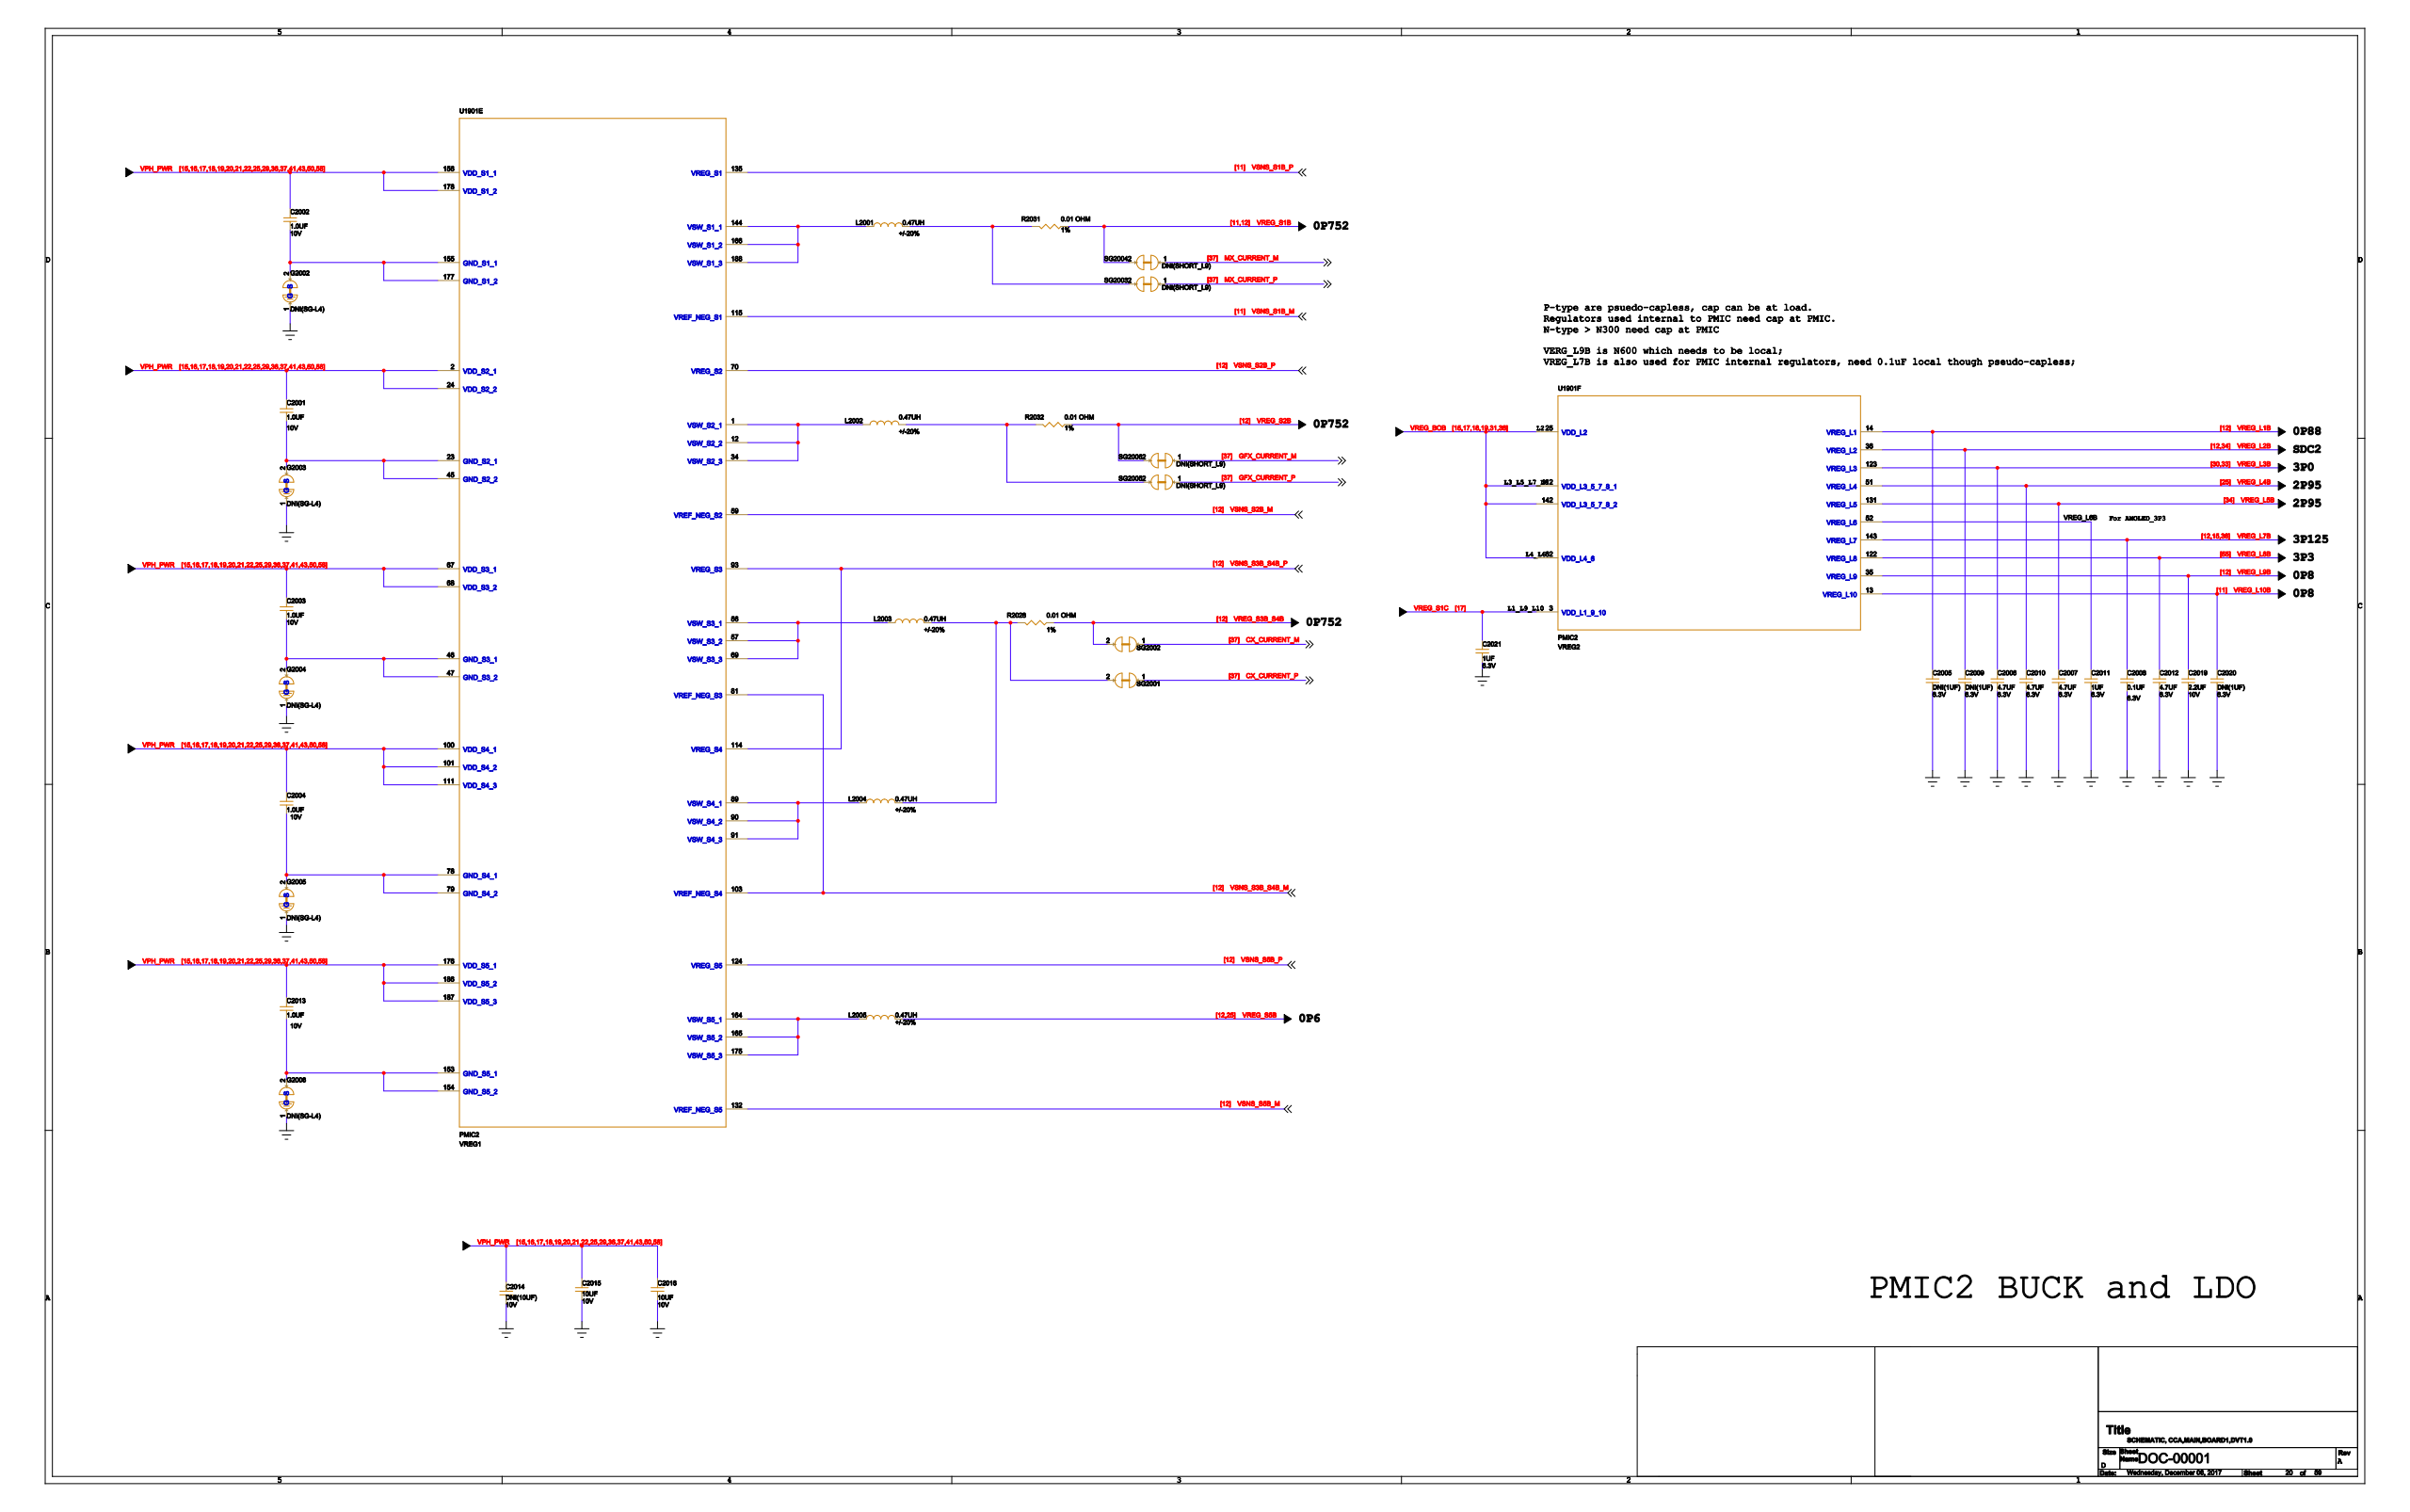Circuit board | KiCad | 1657 parts | 1365 nets | one sheet of the schematic
Parts on this sheet (reference | value | footprint):
C2001
C2002
C2003
C2004
C2005
C2006
C2007
C2008
C2009
C2010
C2011
C2012
C2013
C2014
C2015
C2016
C2019
C2020
C2021
G2002
G2003
G2004
G2005
G2006
L2001
L2002
L2003
L2004
L2005
R2028
R2031
R2032
SG2001
SG2002
SG2003
SG2004
SG2005
SG2006
U1901
Nets of these parts (net: part-pin ...):
GND: C2005-1 C2006-1 C2007-1 C2008-1 C2009-1 C2010-1 C2011-1 C2012-1 C2014-1 C2015-1 C2016-1 C2019-1 C2020-1 C2021-2 G2002-1 G2003-1 G2004-1 G2005-1 G2006-1
VPH_PWR: C2001-2 C2002-2 C2003-2 C2004-2 C2013-2 C2014-2 C2015-2 C2016-2 U1901-2 U1901-17 U1901-21 U1901-24 U1901-67 U1901-68 U1901-100 U1901-101 U1901-111 U1901-156 U1901-176 U1901-178 U1901-186 U1901-187
VREG_L2B: C2009-2 U1901-36
VSNS_S3B_S4B_M: U1901-81 U1901-103
VREG_BOB: U1901-20 U1901-25 U1901-41 U1901-62 U1901-112 U1901-142
VREG_L8B: C2012-2 U1901-122
VREG_S2B: R2032-2 SG2006-2
VSNS_S2B_P: U1901-70
VREG_L7B: C2008-2 U1901-143
N41047485: C2001-1 G2003-2 U1901-23 U1901-45
VREG_L5B: C2007-2 U1901-131
CX_CURRENT_M: SG2002-1
VREG_S3B_S4B: R2028-2 SG2002-2
VSNS_S1B_M: U1901-115
CX_CURRENT_P: SG2001-1
N22195111: L2003-2 L2004-2 R2028-1 SG2001-2
VREG_L4B: C2010-2 U1901-51
VREG_L10B: C2020-2 U1901-13
N41047633: C2003-1 G2004-2 U1901-46 U1901-47
VSNS_S5B_M: U1901-132
N41047782: C2013-1 G2006-2 U1901-153 U1901-154
N41047058: C2002-1 G2002-2 U1901-155 U1901-177
GFX_CURRENT_M: SG2006-1
VSNS_S2B_M: U1901-59
VREG_S1C: C2021-1 U1901-3
VREG_L1B: C2005-2 U1901-14
VREG_S1B: R2031-2 SG2004-2
VREG_S5B: L2005-2
MX_CURRENT_M: SG2004-1
VREG_L3B: C2006-2 U1901-123
N41047701: C2004-1 G2005-2 U1901-78 U1901-79
VSNS_S3B_S4B_P: U1901-93 U1901-114
VSNS_S1B_P: U1901-135
MX_CURRENT_P: SG2003-1
N22194731: L2001-2 R2031-1 SG2003-2
GFX_CURRENT_P: SG2005-1
N22217190: L2002-2 R2032-1 SG2005-2
VREG_L9B: C2019-2 U1901-35
VSNS_S5B_P: U1901-124
N41048843: L2002-1 U1901-1 U1901-12 U1901-34
N41049020: L2003-1 U1901-56 U1901-57 U1901-69
N41048515: L2001-1 U1901-144 U1901-166 U1901-188
VREG_L6B: C2011-2 U1901-52
N41049260: L2004-1 U1901-89 U1901-90 U1901-91
N41049519: L2005-1 U1901-164 U1901-165 U1901-175